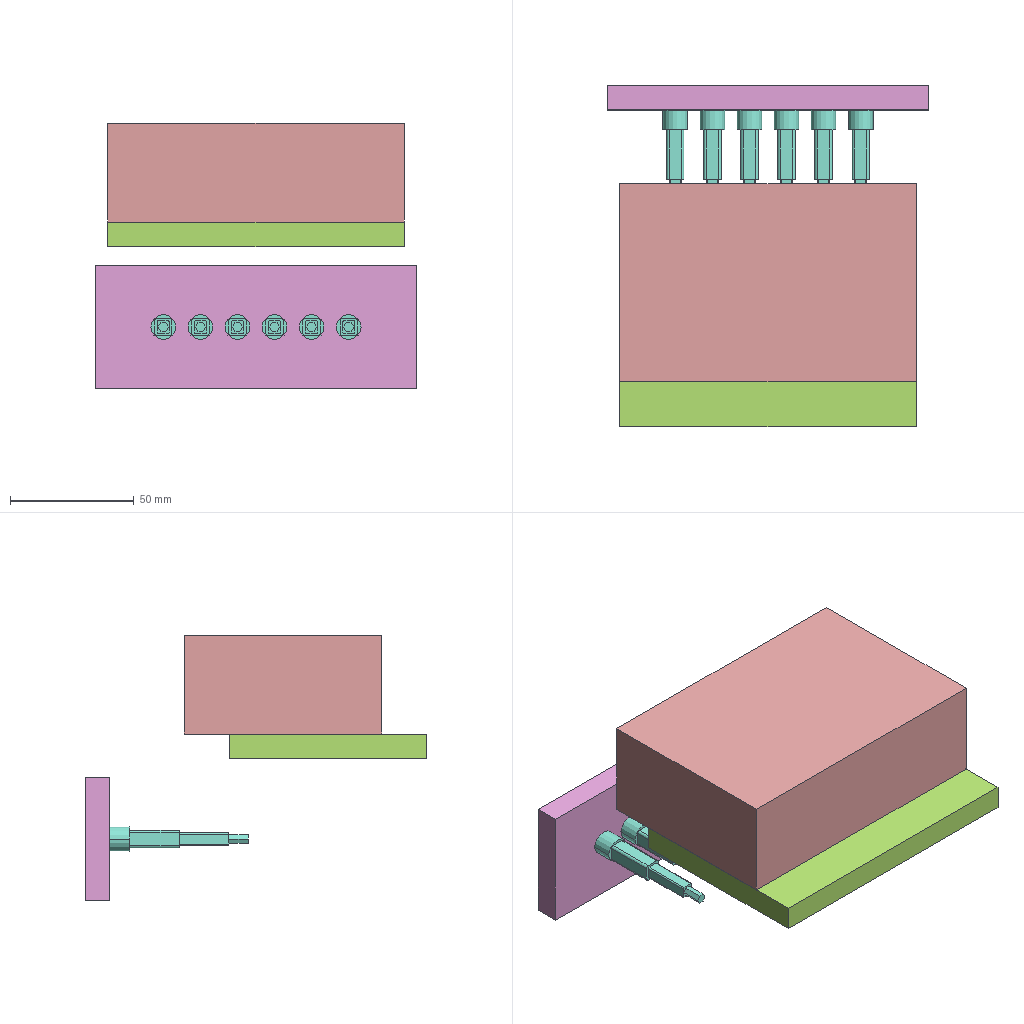Assembly | SolidWorks | 5 different items | 10 placed | box 130 x 138 x 108 mm
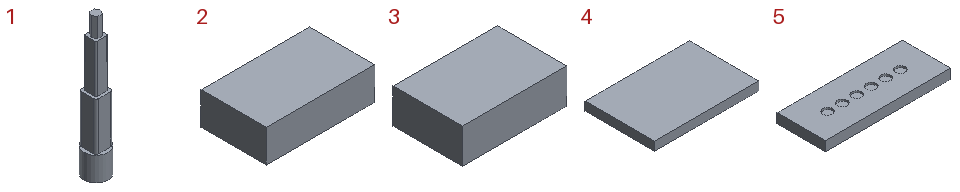Parts list (item | quantity | size | volume | features):
1 | x6 | 10 x 10 x 58 mm | 2347 mm3 | features ICE 3, Fillet 2, Extrusion 1
2 | x1 | 100 x 60 x 30 mm | 180000 mm3 | features Extrusion 1
3 | x1 | 120 x 80 x 40 mm | 204000 mm3 | features ICE 2, Extrusion 1
4 | x1 | 120 x 80 x 10 mm | 96000 mm3 | features ICE 4, Extrusion 1
5 | x1 | 130 x 50 x 10 mm | 64058 mm3 | features Extrusion 1, ICE 1
Mates (type | each side: item.copy, entity, surface, feature):
Coincident | 3.1 face plane Boss-Extrude2 | 2.1 face plane Boss-Extrude1 | 2 times
Coincident | 3.1 face plane Boss-Extrude3 | 2.1 face plane Boss-Extrude1
Coincident | 2.1 face plane Boss-Extrude1 | 4.1 face plane Boss-Extrude4
Coincident | 3.1 face plane Boss-Extrude2 | 4.1 face plane Boss-Extrude4
DistanceDim | 3.1 face plane Boss-Extrude2 | 5.1 face plane Boss-Extrude1 | 2 times
Parallel | 3.1 face plane Boss-Extrude2 | 5.1 face plane Boss-Extrude1
Coincident | 5.1 face plane Cut-Extrude1 | 1.1 face plane Boss-Extrude1
Concentric | 5.1 face cylinder Cut-Extrude1 | 1.1 face cylinder Boss-Extrude1
Coincident | 5.1 face plane Cut-Extrude1 | 1.2 face plane Boss-Extrude1
Coincident | 5.1 edge | 1.2 face cylinder Boss-Extrude1
Coincident | 5.1 face plane Cut-Extrude1 | 1.3 face plane Boss-Extrude1
Coincident | 5.1 edge | 1.3 face cylinder Boss-Extrude1
Coincident | 5.1 face plane Cut-Extrude1 | 1.4 face plane Boss-Extrude1
Coincident | 5.1 edge | 1.4 face cylinder Boss-Extrude1
Coincident | 5.1 face plane Cut-Extrude1 | 1.5 face plane Boss-Extrude1
Coincident | 5.1 edge | 1.5 face cylinder Boss-Extrude1
Coincident | 5.1 face plane Cut-Extrude1 | 1.6 face plane Boss-Extrude1
Coincident | 5.1 edge | 1.6 face cylinder Boss-Extrude1